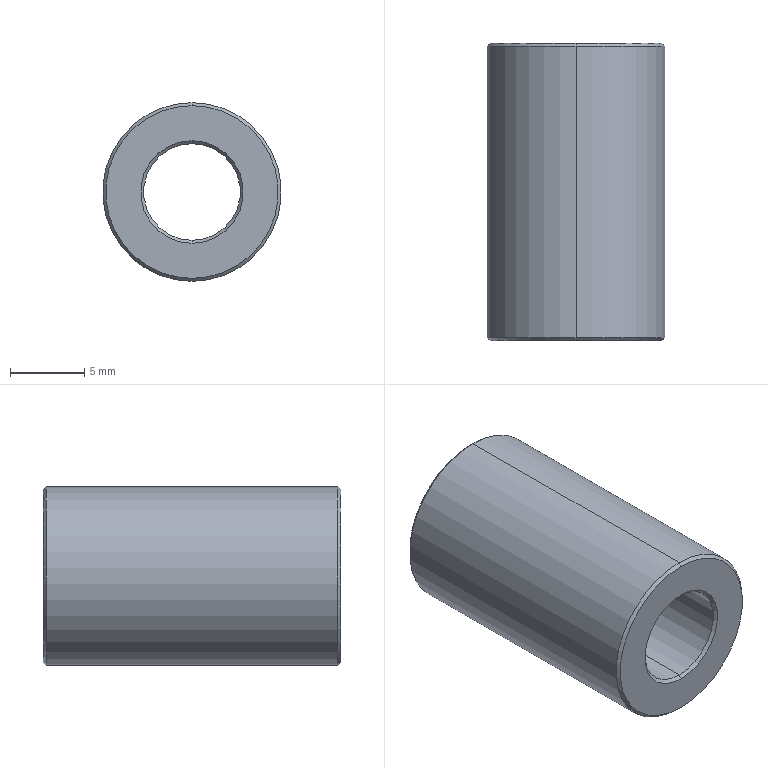Part | STEP file | PN_0025 lifting air cylinder extension rod_Default | 1 solid | 14 faces | box 12 x 20 x 12 mm | volume 1596 mm3 | cone 8 | cylinder 4 | plane 2 | commonest cylinder face diameters 6.5 x2 12 x2
STEP:
#1=CARTESIAN_POINT('',(0.,0.,0.));
#2=DIRECTION('',(0.,0.,1.));
#3=DIRECTION('',(1.,0.,0.));
#4=AXIS2_PLACEMENT_3D('',#1,#2,#3);
#5=CARTESIAN_POINT('',(0.,0.2,-3.25));
#6=VERTEX_POINT('',#5);
#7=CARTESIAN_POINT('',(0.,0.,-3.45));
#8=VERTEX_POINT('',#7);
#9=CARTESIAN_POINT('',(0.,0.,-3.45));
#10=DIRECTION('',(0.,-0.7071,-0.7071));
#11=VECTOR('',#10,1.);
#12=LINE('',#9,#11);
#13=CARTESIAN_POINT('',(0.,0.,0.));
#14=DIRECTION('',(0.,-1.,0.));
#15=DIRECTION('',(0.,0.,-1.));
#16=AXIS2_PLACEMENT_3D('',#13,#14,#15);
#17=CONICAL_SURFACE('',#16,3.45,0.7854);
#18=CARTESIAN_POINT('',(6.283,0.));
#19=DIRECTION('',(0.,1.));
#20=VECTOR('',#19,1.);
#21=LINE('',#18,#20);
#22=(GEOMETRIC_REPRESENTATION_CONTEXT(2)PARAMETRIC_REPRESENTATION_CONTEXT()REPRESENTATION_CONTEXT('',''));
#23=DEFINITIONAL_REPRESENTATION('',(#21),#22);
#24=PCURVE('',#17,#23);
#25=CARTESIAN_POINT('',(0.,0.,0.));
#26=DIRECTION('',(0.,-1.,0.));
#27=DIRECTION('',(0.,0.,-1.));
#28=AXIS2_PLACEMENT_3D('',#25,#26,#27);
#29=CONICAL_SURFACE('',#28,3.45,0.7854);
#30=CARTESIAN_POINT('',(0.,0.));
#31=DIRECTION('',(0.,1.));
#32=VECTOR('',#31,1.);
#33=LINE('',#30,#32);
#34=(GEOMETRIC_REPRESENTATION_CONTEXT(2)PARAMETRIC_REPRESENTATION_CONTEXT()REPRESENTATION_CONTEXT('',''));
#35=DEFINITIONAL_REPRESENTATION('',(#33),#34);
#36=PCURVE('',#29,#35);
#37=SURFACE_CURVE('',#12,(#24,#36),.PCURVE_S1.);
#38=EDGE_CURVE('',#6,#8,#37,.T.);
#39=ORIENTED_EDGE('',*,*,#38,.T.);
#40=CARTESIAN_POINT('',(0.,0.,3.45));
#41=VERTEX_POINT('',#40);
#42=CARTESIAN_POINT('',(0.,0.,0.));
#43=DIRECTION('',(0.,1.,0.));
#44=DIRECTION('',(0.,0.,1.));
#45=AXIS2_PLACEMENT_3D('',#42,#43,#44);
#46=CIRCLE('',#45,3.45);
#47=CARTESIAN_POINT('',(9.425,0.));
#48=DIRECTION('',(-1.,0.));
#49=VECTOR('',#48,1.);
#50=LINE('',#47,#49);
#51=(GEOMETRIC_REPRESENTATION_CONTEXT(2)PARAMETRIC_REPRESENTATION_CONTEXT()REPRESENTATION_CONTEXT('',''));
#52=DEFINITIONAL_REPRESENTATION('',(#50),#51);
#53=PCURVE('',#17,#52);
#54=CARTESIAN_POINT('',(0.,0.,0.));
#55=DIRECTION('',(0.,1.,0.));
#56=DIRECTION('',(0.,0.,1.));
#57=AXIS2_PLACEMENT_3D('',#54,#55,#56);
#58=PLANE('',#57);
#59=CARTESIAN_POINT('',(0.,0.));
#60=DIRECTION('',(1.,0.));
#61=AXIS2_PLACEMENT_2D('',#59,#60);
#62=CIRCLE('',#61,3.45);
#63=(GEOMETRIC_REPRESENTATION_CONTEXT(2)PARAMETRIC_REPRESENTATION_CONTEXT()REPRESENTATION_CONTEXT('',''));
#64=DEFINITIONAL_REPRESENTATION('',(#62),#63);
#65=PCURVE('',#58,#64);
#66=SURFACE_CURVE('',#46,(#53,#65),.PCURVE_S1.);
#67=EDGE_CURVE('',#8,#41,#66,.T.);
#68=ORIENTED_EDGE('',*,*,#67,.T.);
#69=CARTESIAN_POINT('',(0.,0.2,3.25));
#70=VERTEX_POINT('',#69);
#71=CARTESIAN_POINT('',(0.,0.,3.45));
#72=DIRECTION('',(0.,-0.7071,0.7071));
#73=VECTOR('',#72,1.);
#74=LINE('',#71,#73);
#75=CARTESIAN_POINT('',(3.142,0.));
#76=DIRECTION('',(0.,1.));
#77=VECTOR('',#76,1.);
#78=LINE('',#75,#77);
#79=(GEOMETRIC_REPRESENTATION_CONTEXT(2)PARAMETRIC_REPRESENTATION_CONTEXT()REPRESENTATION_CONTEXT('',''));
#80=DEFINITIONAL_REPRESENTATION('',(#78),#79);
#81=PCURVE('',#17,#80);
#82=CARTESIAN_POINT('',(3.142,0.));
#83=DIRECTION('',(0.,1.));
#84=VECTOR('',#83,1.);
#85=LINE('',#82,#84);
#86=(GEOMETRIC_REPRESENTATION_CONTEXT(2)PARAMETRIC_REPRESENTATION_CONTEXT()REPRESENTATION_CONTEXT('',''));
#87=DEFINITIONAL_REPRESENTATION('',(#85),#86);
#88=PCURVE('',#29,#87);
#89=SURFACE_CURVE('',#74,(#81,#88),.PCURVE_S1.);
#90=EDGE_CURVE('',#70,#41,#89,.T.);
#91=ORIENTED_EDGE('',*,*,#90,.F.);
#92=CARTESIAN_POINT('',(0.,0.2,0.));
#93=DIRECTION('',(0.,-1.,0.));
#94=DIRECTION('',(0.,0.,1.));
#95=AXIS2_PLACEMENT_3D('',#92,#93,#94);
#96=CIRCLE('',#95,3.25);
#97=CARTESIAN_POINT('',(3.142,-0.2));
#98=DIRECTION('',(1.,0.));
#99=VECTOR('',#98,1.);
#100=LINE('',#97,#99);
#101=(GEOMETRIC_REPRESENTATION_CONTEXT(2)PARAMETRIC_REPRESENTATION_CONTEXT()REPRESENTATION_CONTEXT('',''));
#102=DEFINITIONAL_REPRESENTATION('',(#100),#101);
#103=PCURVE('',#17,#102);
#104=CARTESIAN_POINT('',(0.,20.,0.));
#105=DIRECTION('',(0.,-1.,0.));
#106=DIRECTION('',(0.,0.,-1.));
#107=AXIS2_PLACEMENT_3D('',#104,#105,#106);
#108=CYLINDRICAL_SURFACE('',#107,3.25);
#109=CARTESIAN_POINT('',(3.142,19.8));
#110=DIRECTION('',(1.,0.));
#111=VECTOR('',#110,1.);
#112=LINE('',#109,#111);
#113=(GEOMETRIC_REPRESENTATION_CONTEXT(2)PARAMETRIC_REPRESENTATION_CONTEXT()REPRESENTATION_CONTEXT('',''));
#114=DEFINITIONAL_REPRESENTATION('',(#112),#113);
#115=PCURVE('',#108,#114);
#116=SURFACE_CURVE('',#96,(#103,#115),.PCURVE_S1.);
#117=EDGE_CURVE('',#70,#6,#116,.T.);
#118=ORIENTED_EDGE('',*,*,#117,.T.);
#119=EDGE_LOOP('',(#39,#68,#91,#118));
#120=FACE_BOUND('',#119,.F.);
#121=ADVANCED_FACE('',(#120),#17,.F.);
#122=CARTESIAN_POINT('',(0.,19.8,3.25));
#123=VERTEX_POINT('',#122);
#124=CARTESIAN_POINT('',(0.,20.,3.45));
#125=VERTEX_POINT('',#124);
#126=CARTESIAN_POINT('',(0.,19.8,3.25));
#127=DIRECTION('',(0.,0.7071,0.7071));
#128=VECTOR('',#127,1.);
#129=LINE('',#126,#128);
#130=CARTESIAN_POINT('',(0.,19.8,0.));
#131=DIRECTION('',(0.,1.,0.));
#132=DIRECTION('',(0.,0.,1.));
#133=AXIS2_PLACEMENT_3D('',#130,#131,#132);
#134=CONICAL_SURFACE('',#133,3.25,0.7854);
#135=CARTESIAN_POINT('',(6.283,0.));
#136=DIRECTION('',(0.,1.));
#137=VECTOR('',#136,1.);
#138=LINE('',#135,#137);
#139=(GEOMETRIC_REPRESENTATION_CONTEXT(2)PARAMETRIC_REPRESENTATION_CONTEXT()REPRESENTATION_CONTEXT('',''));
#140=DEFINITIONAL_REPRESENTATION('',(#138),#139);
#141=PCURVE('',#134,#140);
#142=CARTESIAN_POINT('',(0.,19.8,0.));
#143=DIRECTION('',(0.,1.,0.));
#144=DIRECTION('',(0.,0.,1.));
#145=AXIS2_PLACEMENT_3D('',#142,#143,#144);
#146=CONICAL_SURFACE('',#145,3.25,0.7854);
#147=CARTESIAN_POINT('',(0.,0.));
#148=DIRECTION('',(0.,1.));
#149=VECTOR('',#148,1.);
#150=LINE('',#147,#149);
#151=(GEOMETRIC_REPRESENTATION_CONTEXT(2)PARAMETRIC_REPRESENTATION_CONTEXT()REPRESENTATION_CONTEXT('',''));
#152=DEFINITIONAL_REPRESENTATION('',(#150),#151);
#153=PCURVE('',#146,#152);
#154=SURFACE_CURVE('',#129,(#141,#153),.PCURVE_S1.);
#155=EDGE_CURVE('',#123,#125,#154,.T.);
#156=ORIENTED_EDGE('',*,*,#155,.T.);
#157=CARTESIAN_POINT('',(0.,20.,-3.45));
#158=VERTEX_POINT('',#157);
#159=CARTESIAN_POINT('',(0.,20.,0.));
#160=DIRECTION('',(0.,-1.,0.));
#161=DIRECTION('',(0.,0.,1.));
#162=AXIS2_PLACEMENT_3D('',#159,#160,#161);
#163=CIRCLE('',#162,3.45);
#164=CARTESIAN_POINT('',(6.283,0.2));
#165=DIRECTION('',(-1.,0.));
#166=VECTOR('',#165,1.);
#167=LINE('',#164,#166);
#168=(GEOMETRIC_REPRESENTATION_CONTEXT(2)PARAMETRIC_REPRESENTATION_CONTEXT()REPRESENTATION_CONTEXT('',''));
#169=DEFINITIONAL_REPRESENTATION('',(#167),#168);
#170=PCURVE('',#134,#169);
#171=CARTESIAN_POINT('',(0.,20.,0.));
#172=DIRECTION('',(0.,1.,0.));
#173=DIRECTION('',(0.,0.,1.));
#174=AXIS2_PLACEMENT_3D('',#171,#172,#173);
#175=PLANE('',#174);
#176=CARTESIAN_POINT('',(3.45,0.));
#177=CARTESIAN_POINT('',(3.45,-5.976));
#178=CARTESIAN_POINT('',(-1.725,-2.988));
#179=CARTESIAN_POINT('',(-6.9,0.));
#180=CARTESIAN_POINT('',(-1.725,2.988));
#181=CARTESIAN_POINT('',(3.45,5.976));
#182=CARTESIAN_POINT('',(3.45,0.));
#183=(BOUNDED_CURVE()B_SPLINE_CURVE(2,(#176,#177,#178,#179,#180,#181,#182),.UNSPECIFIED.,.T.,.F.)B_SPLINE_CURVE_WITH_KNOTS((1,2,2,2,2,1),(-2.094,0.,2.094,4.189,6.283,8.378),.UNSPECIFIED.)CURVE()GEOMETRIC_REPRESENTATION_ITEM()RATIONAL_B_SPLINE_CURVE((1.,0.5,1.,0.5,1.,0.5,1.))REPRESENTATION_ITEM(''));
#184=(GEOMETRIC_REPRESENTATION_CONTEXT(2)PARAMETRIC_REPRESENTATION_CONTEXT()REPRESENTATION_CONTEXT('',''));
#185=DEFINITIONAL_REPRESENTATION('',(#183),#184);
#186=PCURVE('',#175,#185);
#187=SURFACE_CURVE('',#163,(#170,#186),.PCURVE_S1.);
#188=EDGE_CURVE('',#125,#158,#187,.T.);
#189=ORIENTED_EDGE('',*,*,#188,.T.);
#190=CARTESIAN_POINT('',(0.,19.8,-3.25));
#191=VERTEX_POINT('',#190);
#192=CARTESIAN_POINT('',(0.,19.8,-3.25));
#193=DIRECTION('',(0.,0.7071,-0.7071));
#194=VECTOR('',#193,1.);
#195=LINE('',#192,#194);
#196=CARTESIAN_POINT('',(3.142,0.));
#197=DIRECTION('',(0.,1.));
#198=VECTOR('',#197,1.);
#199=LINE('',#196,#198);
#200=(GEOMETRIC_REPRESENTATION_CONTEXT(2)PARAMETRIC_REPRESENTATION_CONTEXT()REPRESENTATION_CONTEXT('',''));
#201=DEFINITIONAL_REPRESENTATION('',(#199),#200);
#202=PCURVE('',#134,#201);
#203=CARTESIAN_POINT('',(3.142,0.));
#204=DIRECTION('',(0.,1.));
#205=VECTOR('',#204,1.);
#206=LINE('',#203,#205);
#207=(GEOMETRIC_REPRESENTATION_CONTEXT(2)PARAMETRIC_REPRESENTATION_CONTEXT()REPRESENTATION_CONTEXT('',''));
#208=DEFINITIONAL_REPRESENTATION('',(#206),#207);
#209=PCURVE('',#146,#208);
#210=SURFACE_CURVE('',#195,(#202,#209),.PCURVE_S1.);
#211=EDGE_CURVE('',#191,#158,#210,.T.);
#212=ORIENTED_EDGE('',*,*,#211,.F.);
#213=CARTESIAN_POINT('',(0.,19.8,0.));
#214=DIRECTION('',(0.,1.,0.));
#215=DIRECTION('',(0.,0.,1.));
#216=AXIS2_PLACEMENT_3D('',#213,#214,#215);
#217=CIRCLE('',#216,3.25);
#218=CARTESIAN_POINT('',(0.,0.));
#219=DIRECTION('',(1.,0.));
#220=VECTOR('',#219,1.);
#221=LINE('',#218,#220);
#222=(GEOMETRIC_REPRESENTATION_CONTEXT(2)PARAMETRIC_REPRESENTATION_CONTEXT()REPRESENTATION_CONTEXT('',''));
#223=DEFINITIONAL_REPRESENTATION('',(#221),#222);
#224=PCURVE('',#134,#223);
#225=CARTESIAN_POINT('',(9.425,0.2));
#226=DIRECTION('',(-1.,0.));
#227=VECTOR('',#226,1.);
#228=LINE('',#225,#227);
#229=(GEOMETRIC_REPRESENTATION_CONTEXT(2)PARAMETRIC_REPRESENTATION_CONTEXT()REPRESENTATION_CONTEXT('',''));
#230=DEFINITIONAL_REPRESENTATION('',(#228),#229);
#231=PCURVE('',#108,#230);
#232=SURFACE_CURVE('',#217,(#224,#231),.PCURVE_S1.);
#233=EDGE_CURVE('',#191,#123,#232,.T.);
#234=ORIENTED_EDGE('',*,*,#233,.T.);
#235=EDGE_LOOP('',(#156,#189,#212,#234));
#236=FACE_BOUND('',#235,.F.);
#237=ADVANCED_FACE('',(#236),#134,.F.);
#238=CARTESIAN_POINT('',(0.,0.,-5.8));
#239=VERTEX_POINT('',#238);
#240=CARTESIAN_POINT('',(0.,0.,5.8));
#241=VERTEX_POINT('',#240);
#242=CARTESIAN_POINT('',(0.,0.,0.));
#243=DIRECTION('',(0.,-1.,0.));
#244=DIRECTION('',(0.,0.,1.));
#245=AXIS2_PLACEMENT_3D('',#242,#243,#244);
#246=CIRCLE('',#245,5.8);
#247=CARTESIAN_POINT('',(0.,0.2,0.));
#248=DIRECTION('',(0.,1.,0.));
#249=DIRECTION('',(0.,0.,1.));
#250=AXIS2_PLACEMENT_3D('',#247,#248,#249);
#251=CONICAL_SURFACE('',#250,6.,0.7854);
#252=CARTESIAN_POINT('',(6.283,-0.2));
#253=DIRECTION('',(-1.,0.));
#254=VECTOR('',#253,1.);
#255=LINE('',#252,#254);
#256=(GEOMETRIC_REPRESENTATION_CONTEXT(2)PARAMETRIC_REPRESENTATION_CONTEXT()REPRESENTATION_CONTEXT('',''));
#257=DEFINITIONAL_REPRESENTATION('',(#255),#256);
#258=PCURVE('',#251,#257);
#259=CARTESIAN_POINT('',(5.8,0.));
#260=CARTESIAN_POINT('',(5.8,-10.046));
#261=CARTESIAN_POINT('',(-2.9,-5.023));
#262=CARTESIAN_POINT('',(-11.6,0.));
#263=CARTESIAN_POINT('',(-2.9,5.023));
#264=CARTESIAN_POINT('',(5.8,10.046));
#265=CARTESIAN_POINT('',(5.8,0.));
#266=(BOUNDED_CURVE()B_SPLINE_CURVE(2,(#259,#260,#261,#262,#263,#264,#265),.UNSPECIFIED.,.T.,.F.)B_SPLINE_CURVE_WITH_KNOTS((1,2,2,2,2,1),(-2.094,0.,2.094,4.189,6.283,8.378),.UNSPECIFIED.)CURVE()GEOMETRIC_REPRESENTATION_ITEM()RATIONAL_B_SPLINE_CURVE((1.,0.5,1.,0.5,1.,0.5,1.))REPRESENTATION_ITEM(''));
#267=(GEOMETRIC_REPRESENTATION_CONTEXT(2)PARAMETRIC_REPRESENTATION_CONTEXT()REPRESENTATION_CONTEXT('',''));
#268=DEFINITIONAL_REPRESENTATION('',(#266),#267);
#269=PCURVE('',#58,#268);
#270=SURFACE_CURVE('',#246,(#258,#269),.PCURVE_S1.);
#271=EDGE_CURVE('',#239,#241,#270,.T.);
#272=ORIENTED_EDGE('',*,*,#271,.F.);
#273=CARTESIAN_POINT('',(0.,0.2,-6.));
#274=VERTEX_POINT('',#273);
#275=CARTESIAN_POINT('',(0.,0.2,-6.));
#276=DIRECTION('',(0.,0.7071,-0.7071));
#277=VECTOR('',#276,1.);
#278=LINE('',#275,#277);
#279=CARTESIAN_POINT('',(3.142,0.));
#280=DIRECTION('',(0.,1.));
#281=VECTOR('',#280,1.);
#282=LINE('',#279,#281);
#283=(GEOMETRIC_REPRESENTATION_CONTEXT(2)PARAMETRIC_REPRESENTATION_CONTEXT()REPRESENTATION_CONTEXT('',''));
#284=DEFINITIONAL_REPRESENTATION('',(#282),#283);
#285=PCURVE('',#251,#284);
#286=CARTESIAN_POINT('',(0.,0.2,0.));
#287=DIRECTION('',(0.,1.,0.));
#288=DIRECTION('',(0.,0.,1.));
#289=AXIS2_PLACEMENT_3D('',#286,#287,#288);
#290=CONICAL_SURFACE('',#289,6.,0.7854);
#291=CARTESIAN_POINT('',(3.142,0.));
#292=DIRECTION('',(0.,1.));
#293=VECTOR('',#292,1.);
#294=LINE('',#291,#293);
#295=(GEOMETRIC_REPRESENTATION_CONTEXT(2)PARAMETRIC_REPRESENTATION_CONTEXT()REPRESENTATION_CONTEXT('',''));
#296=DEFINITIONAL_REPRESENTATION('',(#294),#295);
#297=PCURVE('',#290,#296);
#298=SURFACE_CURVE('',#278,(#285,#297),.PCURVE_S1.);
#299=EDGE_CURVE('',#239,#274,#298,.T.);
#300=ORIENTED_EDGE('',*,*,#299,.T.);
#301=CARTESIAN_POINT('',(0.,0.2,6.));
#302=VERTEX_POINT('',#301);
#303=CARTESIAN_POINT('',(0.,0.2,0.));
#304=DIRECTION('',(0.,1.,0.));
#305=DIRECTION('',(0.,0.,1.));
#306=AXIS2_PLACEMENT_3D('',#303,#304,#305);
#307=CIRCLE('',#306,6.);
#308=CARTESIAN_POINT('',(0.,0.));
#309=DIRECTION('',(1.,0.));
#310=VECTOR('',#309,1.);
#311=LINE('',#308,#310);
#312=(GEOMETRIC_REPRESENTATION_CONTEXT(2)PARAMETRIC_REPRESENTATION_CONTEXT()REPRESENTATION_CONTEXT('',''));
#313=DEFINITIONAL_REPRESENTATION('',(#311),#312);
#314=PCURVE('',#251,#313);
#315=CARTESIAN_POINT('',(0.,20.,0.));
#316=DIRECTION('',(0.,-1.,0.));
#317=DIRECTION('',(0.,0.,-1.));
#318=AXIS2_PLACEMENT_3D('',#315,#316,#317);
#319=CYLINDRICAL_SURFACE('',#318,6.);
#320=CARTESIAN_POINT('',(3.142,19.8));
#321=DIRECTION('',(-1.,0.));
#322=VECTOR('',#321,1.);
#323=LINE('',#320,#322);
#324=(GEOMETRIC_REPRESENTATION_CONTEXT(2)PARAMETRIC_REPRESENTATION_CONTEXT()REPRESENTATION_CONTEXT('',''));
#325=DEFINITIONAL_REPRESENTATION('',(#323),#324);
#326=PCURVE('',#319,#325);
#327=SURFACE_CURVE('',#307,(#314,#326),.PCURVE_S1.);
#328=EDGE_CURVE('',#302,#274,#327,.T.);
#329=ORIENTED_EDGE('',*,*,#328,.F.);
#330=CARTESIAN_POINT('',(0.,0.2,6.));
#331=DIRECTION('',(0.,0.7071,0.7071));
#332=VECTOR('',#331,1.);
#333=LINE('',#330,#332);
#334=CARTESIAN_POINT('',(0.,0.));
#335=DIRECTION('',(0.,1.));
#336=VECTOR('',#335,1.);
#337=LINE('',#334,#336);
#338=(GEOMETRIC_REPRESENTATION_CONTEXT(2)PARAMETRIC_REPRESENTATION_CONTEXT()REPRESENTATION_CONTEXT('',''));
#339=DEFINITIONAL_REPRESENTATION('',(#337),#338);
#340=PCURVE('',#251,#339);
#341=CARTESIAN_POINT('',(6.283,0.));
#342=DIRECTION('',(0.,1.));
#343=VECTOR('',#342,1.);
#344=LINE('',#341,#343);
#345=(GEOMETRIC_REPRESENTATION_CONTEXT(2)PARAMETRIC_REPRESENTATION_CONTEXT()REPRESENTATION_CONTEXT('',''));
#346=DEFINITIONAL_REPRESENTATION('',(#344),#345);
#347=PCURVE('',#290,#346);
#348=SURFACE_CURVE('',#333,(#340,#347),.PCURVE_S1.);
#349=EDGE_CURVE('',#241,#302,#348,.T.);
#350=ORIENTED_EDGE('',*,*,#349,.F.);
#351=EDGE_LOOP('',(#272,#300,#329,#350));
#352=FACE_BOUND('',#351,.T.);
#353=ADVANCED_FACE('',(#352),#251,.T.);
#354=CARTESIAN_POINT('',(0.,20.,5.8));
#355=VERTEX_POINT('',#354);
#356=CARTESIAN_POINT('',(0.,20.,-5.8));
#357=VERTEX_POINT('',#356);
#358=CARTESIAN_POINT('',(0.,20.,0.));
#359=DIRECTION('',(0.,1.,0.));
#360=DIRECTION('',(0.,0.,1.));
#361=AXIS2_PLACEMENT_3D('',#358,#359,#360);
#362=CIRCLE('',#361,5.8);
#363=CARTESIAN_POINT('',(0.,20.,0.));
#364=DIRECTION('',(0.,-1.,0.));
#365=DIRECTION('',(0.,0.,-1.));
#366=AXIS2_PLACEMENT_3D('',#363,#364,#365);
#367=CONICAL_SURFACE('',#366,5.8,0.7854);
#368=CARTESIAN_POINT('',(3.142,0.));
#369=DIRECTION('',(-1.,0.));
#370=VECTOR('',#369,1.);
#371=LINE('',#368,#370);
#372=(GEOMETRIC_REPRESENTATION_CONTEXT(2)PARAMETRIC_REPRESENTATION_CONTEXT()REPRESENTATION_CONTEXT('',''));
#373=DEFINITIONAL_REPRESENTATION('',(#371),#372);
#374=PCURVE('',#367,#373);
#375=CARTESIAN_POINT('',(0.,0.));
#376=DIRECTION('',(1.,0.));
#377=AXIS2_PLACEMENT_2D('',#375,#376);
#378=CIRCLE('',#377,5.8);
#379=(GEOMETRIC_REPRESENTATION_CONTEXT(2)PARAMETRIC_REPRESENTATION_CONTEXT()REPRESENTATION_CONTEXT('',''));
#380=DEFINITIONAL_REPRESENTATION('',(#378),#379);
#381=PCURVE('',#175,#380);
#382=SURFACE_CURVE('',#362,(#374,#381),.PCURVE_S1.);
#383=EDGE_CURVE('',#355,#357,#382,.T.);
#384=ORIENTED_EDGE('',*,*,#383,.F.);
#385=CARTESIAN_POINT('',(0.,19.8,6.));
#386=VERTEX_POINT('',#385);
#387=CARTESIAN_POINT('',(0.,20.,5.8));
#388=DIRECTION('',(0.,-0.7071,0.7071));
#389=VECTOR('',#388,1.);
#390=LINE('',#387,#389);
#391=CARTESIAN_POINT('',(3.142,0.));
#392=DIRECTION('',(0.,1.));
#393=VECTOR('',#392,1.);
#394=LINE('',#391,#393);
#395=(GEOMETRIC_REPRESENTATION_CONTEXT(2)PARAMETRIC_REPRESENTATION_CONTEXT()REPRESENTATION_CONTEXT('',''));
#396=DEFINITIONAL_REPRESENTATION('',(#394),#395);
#397=PCURVE('',#367,#396);
#398=CARTESIAN_POINT('',(0.,20.,0.));
#399=DIRECTION('',(0.,-1.,0.));
#400=DIRECTION('',(0.,0.,-1.));
#401=AXIS2_PLACEMENT_3D('',#398,#399,#400);
#402=CONICAL_SURFACE('',#401,5.8,0.7854);
#403=CARTESIAN_POINT('',(3.142,0.));
#404=DIRECTION('',(0.,1.));
#405=VECTOR('',#404,1.);
#406=LINE('',#403,#405);
#407=(GEOMETRIC_REPRESENTATION_CONTEXT(2)PARAMETRIC_REPRESENTATION_CONTEXT()REPRESENTATION_CONTEXT('',''));
#408=DEFINITIONAL_REPRESENTATION('',(#406),#407);
#409=PCURVE('',#402,#408);
#410=SURFACE_CURVE('',#390,(#397,#409),.PCURVE_S1.);
#411=EDGE_CURVE('',#355,#386,#410,.T.);
#412=ORIENTED_EDGE('',*,*,#411,.T.);
#413=CARTESIAN_POINT('',(0.,19.8,-6.));
#414=VERTEX_POINT('',#413);
#415=CARTESIAN_POINT('',(0.,19.8,0.));
#416=DIRECTION('',(0.,-1.,0.));
#417=DIRECTION('',(0.,0.,1.));
#418=AXIS2_PLACEMENT_3D('',#415,#416,#417);
#419=CIRCLE('',#418,6.);
#420=CARTESIAN_POINT('',(-3.142,0.2));
#421=DIRECTION('',(1.,0.));
#422=VECTOR('',#421,1.);
#423=LINE('',#420,#422);
#424=(GEOMETRIC_REPRESENTATION_CONTEXT(2)PARAMETRIC_REPRESENTATION_CONTEXT()REPRESENTATION_CONTEXT('',''));
#425=DEFINITIONAL_REPRESENTATION('',(#423),#424);
#426=PCURVE('',#367,#425);
#427=CARTESIAN_POINT('',(-3.142,0.2));
#428=DIRECTION('',(1.,0.));
#429=VECTOR('',#428,1.);
#430=LINE('',#427,#429);
#431=(GEOMETRIC_REPRESENTATION_CONTEXT(2)PARAMETRIC_REPRESENTATION_CONTEXT()REPRESENTATION_CONTEXT('',''));
#432=DEFINITIONAL_REPRESENTATION('',(#430),#431);
#433=PCURVE('',#319,#432);
#434=SURFACE_CURVE('',#419,(#426,#433),.PCURVE_S1.);
#435=EDGE_CURVE('',#414,#386,#434,.T.);
#436=ORIENTED_EDGE('',*,*,#435,.F.);
#437=CARTESIAN_POINT('',(0.,20.,-5.8));
#438=DIRECTION('',(0.,-0.7071,-0.7071));
#439=VECTOR('',#438,1.);
#440=LINE('',#437,#439);
#441=CARTESIAN_POINT('',(0.,0.));
#442=DIRECTION('',(0.,1.));
#443=VECTOR('',#442,1.);
#444=LINE('',#441,#443);
#445=(GEOMETRIC_REPRESENTATION_CONTEXT(2)PARAMETRIC_REPRESENTATION_CONTEXT()REPRESENTATION_CONTEXT('',''));
#446=DEFINITIONAL_REPRESENTATION('',(#444),#445);
#447=PCURVE('',#367,#446);
#448=CARTESIAN_POINT('',(6.283,0.));
#449=DIRECTION('',(0.,1.));
#450=VECTOR('',#449,1.);
#451=LINE('',#448,#450);
#452=(GEOMETRIC_REPRESENTATION_CONTEXT(2)PARAMETRIC_REPRESENTATION_CONTEXT()REPRESENTATION_CONTEXT('',''));
#453=DEFINITIONAL_REPRESENTATION('',(#451),#452);
#454=PCURVE('',#402,#453);
#455=SURFACE_CURVE('',#440,(#447,#454),.PCURVE_S1.);
#456=EDGE_CURVE('',#357,#414,#455,.T.);
#457=ORIENTED_EDGE('',*,*,#456,.F.);
#458=EDGE_LOOP('',(#384,#412,#436,#457));
#459=FACE_BOUND('',#458,.T.);
#460=ADVANCED_FACE('',(#459),#367,.T.);
#461=CARTESIAN_POINT('',(0.,20.,-3.25));
#462=DIRECTION('',(0.,-1.,0.));
#463=VECTOR('',#462,1.);
#464=LINE('',#461,#463);
#465=CARTESIAN_POINT('',(6.283,0.));
#466=DIRECTION('',(0.,1.));
#467=VECTOR('',#466,1.);
#468=LINE('',#465,#467);
#469=(GEOMETRIC_REPRESENTATION_CONTEXT(2)PARAMETRIC_REPRESENTATION_CONTEXT()REPRESENTATION_CONTEXT('',''));
#470=DEFINITIONAL_REPRESENTATION('',(#468),#469);
#471=PCURVE('',#108,#470);
#472=CARTESIAN_POINT('',(0.,20.,0.));
#473=DIRECTION('',(0.,-1.,0.));
#474=DIRECTION('',(0.,0.,-1.));
#475=AXIS2_PLACEMENT_3D('',#472,#473,#474);
#476=CYLINDRICAL_SURFACE('',#475,3.25);
#477=CARTESIAN_POINT('',(0.,0.));
#478=DIRECTION('',(0.,1.));
#479=VECTOR('',#478,1.);
#480=LINE('',#477,#479);
#481=(GEOMETRIC_REPRESENTATION_CONTEXT(2)PARAMETRIC_REPRESENTATION_CONTEXT()REPRESENTATION_CONTEXT('',''));
#482=DEFINITIONAL_REPRESENTATION('',(#480),#481);
#483=PCURVE('',#476,#482);
#484=SURFACE_CURVE('',#464,(#471,#483),.PCURVE_S1.);
#485=EDGE_CURVE('',#191,#6,#484,.T.);
#486=ORIENTED_EDGE('',*,*,#485,.T.);
#487=ORIENTED_EDGE('',*,*,#117,.F.);
#488=CARTESIAN_POINT('',(0.,20.,3.25));
#489=DIRECTION('',(0.,-1.,0.));
#490=VECTOR('',#489,1.);
#491=LINE('',#488,#490);
#492=CARTESIAN_POINT('',(3.142,0.));
#493=DIRECTION('',(0.,1.));
#494=VECTOR('',#493,1.);
#495=LINE('',#492,#494);
#496=(GEOMETRIC_REPRESENTATION_CONTEXT(2)PARAMETRIC_REPRESENTATION_CONTEXT()REPRESENTATION_CONTEXT('',''));
#497=DEFINITIONAL_REPRESENTATION('',(#495),#496);
#498=PCURVE('',#108,#497);
#499=CARTESIAN_POINT('',(3.142,0.));
#500=DIRECTION('',(0.,1.));
#501=VECTOR('',#500,1.);
#502=LINE('',#499,#501);
#503=(GEOMETRIC_REPRESENTATION_CONTEXT(2)PARAMETRIC_REPRESENTATION_CONTEXT()REPRESENTATION_CONTEXT('',''));
#504=DEFINITIONAL_REPRESENTATION('',(#502),#503);
#505=PCURVE('',#476,#504);
#506=SURFACE_CURVE('',#491,(#498,#505),.PCURVE_S1.);
#507=EDGE_CURVE('',#123,#70,#506,.T.);
#508=ORIENTED_EDGE('',*,*,#507,.F.);
#509=ORIENTED_EDGE('',*,*,#233,.F.);
#510=EDGE_LOOP('',(#486,#487,#508,#509));
#511=FACE_BOUND('',#510,.F.);
#512=ADVANCED_FACE('',(#511),#108,.F.);
#513=ORIENTED_EDGE('',*,*,#435,.T.);
#514=CARTESIAN_POINT('',(0.,20.,6.));
#515=DIRECTION('',(0.,-1.,0.));
#516=VECTOR('',#515,1.);
#517=LINE('',#514,#516);
#518=CARTESIAN_POINT('',(3.142,0.));
#519=DIRECTION('',(0.,1.));
#520=VECTOR('',#519,1.);
#521=LINE('',#518,#520);
#522=(GEOMETRIC_REPRESENTATION_CONTEXT(2)PARAMETRIC_REPRESENTATION_CONTEXT()REPRESENTATION_CONTEXT('',''));
#523=DEFINITIONAL_REPRESENTATION('',(#521),#522);
#524=PCURVE('',#319,#523);
#525=CARTESIAN_POINT('',(0.,20.,0.));
#526=DIRECTION('',(0.,-1.,0.));
#527=DIRECTION('',(0.,0.,-1.));
#528=AXIS2_PLACEMENT_3D('',#525,#526,#527);
#529=CYLINDRICAL_SURFACE('',#528,6.);
#530=CARTESIAN_POINT('',(3.142,0.));
#531=DIRECTION('',(0.,1.));
#532=VECTOR('',#531,1.);
#533=LINE('',#530,#532);
#534=(GEOMETRIC_REPRESENTATION_CONTEXT(2)PARAMETRIC_REPRESENTATION_CONTEXT()REPRESENTATION_CONTEXT('',''));
#535=DEFINITIONAL_REPRESENTATION('',(#533),#534);
#536=PCURVE('',#529,#535);
#537=SURFACE_CURVE('',#517,(#524,#536),.PCURVE_S1.);
#538=EDGE_CURVE('',#386,#302,#537,.T.);
#539=ORIENTED_EDGE('',*,*,#538,.T.);
#540=ORIENTED_EDGE('',*,*,#328,.T.);
#541=CARTESIAN_POINT('',(0.,20.,-6.));
#542=DIRECTION('',(0.,-1.,0.));
#543=VECTOR('',#542,1.);
#544=LINE('',#541,#543);
#545=CARTESIAN_POINT('',(0.,0.));
#546=DIRECTION('',(0.,1.));
#547=VECTOR('',#546,1.);
#548=LINE('',#545,#547);
#549=(GEOMETRIC_REPRESENTATION_CONTEXT(2)PARAMETRIC_REPRESENTATION_CONTEXT()REPRESENTATION_CONTEXT('',''));
#550=DEFINITIONAL_REPRESENTATION('',(#548),#549);
#551=PCURVE('',#319,#550);
#552=CARTESIAN_POINT('',(6.283,0.));
#553=DIRECTION('',(0.,1.));
#554=VECTOR('',#553,1.);
#555=LINE('',#552,#554);
#556=(GEOMETRIC_REPRESENTATION_CONTEXT(2)PARAMETRIC_REPRESENTATION_CONTEXT()REPRESENTATION_CONTEXT('',''));
#557=DEFINITIONAL_REPRESENTATION('',(#555),#556);
#558=PCURVE('',#529,#557);
#559=SURFACE_CURVE('',#544,(#551,#558),.PCURVE_S1.);
#560=EDGE_CURVE('',#414,#274,#559,.T.);
#561=ORIENTED_EDGE('',*,*,#560,.F.);
#562=EDGE_LOOP('',(#513,#539,#540,#561));
#563=FACE_BOUND('',#562,.T.);
#564=ADVANCED_FACE('',(#563),#319,.T.);
#565=CARTESIAN_POINT('',(0.,20.,0.));
#566=DIRECTION('',(0.,1.,0.));
#567=DIRECTION('',(0.,0.,1.));
#568=AXIS2_PLACEMENT_3D('',#565,#566,#567);
#569=CIRCLE('',#568,5.8);
#570=CARTESIAN_POINT('',(0.,0.));
#571=DIRECTION('',(1.,0.));
#572=AXIS2_PLACEMENT_2D('',#570,#571);
#573=CIRCLE('',#572,5.8);
#574=(GEOMETRIC_REPRESENTATION_CONTEXT(2)PARAMETRIC_REPRESENTATION_CONTEXT()REPRESENTATION_CONTEXT('',''));
#575=DEFINITIONAL_REPRESENTATION('',(#573),#574);
#576=PCURVE('',#175,#575);
#577=CARTESIAN_POINT('',(9.425,0.));
#578=DIRECTION('',(-1.,0.));
#579=VECTOR('',#578,1.);
#580=LINE('',#577,#579);
#581=(GEOMETRIC_REPRESENTATION_CONTEXT(2)PARAMETRIC_REPRESENTATION_CONTEXT()REPRESENTATION_CONTEXT('',''));
#582=DEFINITIONAL_REPRESENTATION('',(#580),#581);
#583=PCURVE('',#402,#582);
#584=SURFACE_CURVE('',#569,(#576,#583),.PCURVE_S1.);
#585=EDGE_CURVE('',#357,#355,#584,.T.);
#586=ORIENTED_EDGE('',*,*,#585,.T.);
#587=ORIENTED_EDGE('',*,*,#383,.T.);
#588=EDGE_LOOP('',(#586,#587));
#589=FACE_BOUND('',#588,.T.);
#590=ORIENTED_EDGE('',*,*,#188,.T.);
#591=CARTESIAN_POINT('',(0.,20.,0.));
#592=DIRECTION('',(0.,-1.,0.));
#593=DIRECTION('',(0.,0.,1.));
#594=AXIS2_PLACEMENT_3D('',#591,#592,#593);
#595=CIRCLE('',#594,3.45);
#596=CARTESIAN_POINT('',(3.45,0.));
#597=CARTESIAN_POINT('',(3.45,-5.976));
#598=CARTESIAN_POINT('',(-1.725,-2.988));
#599=CARTESIAN_POINT('',(-6.9,0.));
#600=CARTESIAN_POINT('',(-1.725,2.988));
#601=CARTESIAN_POINT('',(3.45,5.976));
#602=CARTESIAN_POINT('',(3.45,0.));
#603=(BOUNDED_CURVE()B_SPLINE_CURVE(2,(#596,#597,#598,#599,#600,#601,#602),.UNSPECIFIED.,.T.,.F.)B_SPLINE_CURVE_WITH_KNOTS((1,2,2,2,2,1),(-2.094,0.,2.094,4.189,6.283,8.378),.UNSPECIFIED.)CURVE()GEOMETRIC_REPRESENTATION_ITEM()RATIONAL_B_SPLINE_CURVE((1.,0.5,1.,0.5,1.,0.5,1.))REPRESENTATION_ITEM(''));
#604=(GEOMETRIC_REPRESENTATION_CONTEXT(2)PARAMETRIC_REPRESENTATION_CONTEXT()REPRESENTATION_CONTEXT('',''));
#605=DEFINITIONAL_REPRESENTATION('',(#603),#604);
#606=PCURVE('',#175,#605);
#607=CARTESIAN_POINT('',(6.283,0.2));
#608=DIRECTION('',(-1.,0.));
#609=VECTOR('',#608,1.);
#610=LINE('',#607,#609);
#611=(GEOMETRIC_REPRESENTATION_CONTEXT(2)PARAMETRIC_REPRESENTATION_CONTEXT()REPRESENTATION_CONTEXT('',''));
#612=DEFINITIONAL_REPRESENTATION('',(#610),#611);
#613=PCURVE('',#146,#612);
#614=SURFACE_CURVE('',#595,(#606,#613),.PCURVE_S1.);
#615=EDGE_CURVE('',#158,#125,#614,.T.);
#616=ORIENTED_EDGE('',*,*,#615,.T.);
#617=EDGE_LOOP('',(#590,#616));
#618=FACE_BOUND('',#617,.T.);
#619=ADVANCED_FACE('',(#589,#618),#175,.T.);
#620=CARTESIAN_POINT('',(0.,0.,0.));
#621=DIRECTION('',(0.,-1.,0.));
#622=DIRECTION('',(0.,0.,1.));
#623=AXIS2_PLACEMENT_3D('',#620,#621,#622);
#624=CIRCLE('',#623,5.8);
#625=CARTESIAN_POINT('',(5.8,0.));
#626=CARTESIAN_POINT('',(5.8,-10.046));
#627=CARTESIAN_POINT('',(-2.9,-5.023));
#628=CARTESIAN_POINT('',(-11.6,0.));
#629=CARTESIAN_POINT('',(-2.9,5.023));
#630=CARTESIAN_POINT('',(5.8,10.046));
#631=CARTESIAN_POINT('',(5.8,0.));
#632=(BOUNDED_CURVE()B_SPLINE_CURVE(2,(#625,#626,#627,#628,#629,#630,#631),.UNSPECIFIED.,.T.,.F.)B_SPLINE_CURVE_WITH_KNOTS((1,2,2,2,2,1),(-2.094,0.,2.094,4.189,6.283,8.378),.UNSPECIFIED.)CURVE()GEOMETRIC_REPRESENTATION_ITEM()RATIONAL_B_SPLINE_CURVE((1.,0.5,1.,0.5,1.,0.5,1.))REPRESENTATION_ITEM(''));
#633=(GEOMETRIC_REPRESENTATION_CONTEXT(2)PARAMETRIC_REPRESENTATION_CONTEXT()REPRESENTATION_CONTEXT('',''));
#634=DEFINITIONAL_REPRESENTATION('',(#632),#633);
#635=PCURVE('',#58,#634);
#636=CARTESIAN_POINT('',(6.283,-0.2));
#637=DIRECTION('',(-1.,0.));
#638=VECTOR('',#637,1.);
#639=LINE('',#636,#638);
#640=(GEOMETRIC_REPRESENTATION_CONTEXT(2)PARAMETRIC_REPRESENTATION_CONTEXT()REPRESENTATION_CONTEXT('',''));
#641=DEFINITIONAL_REPRESENTATION('',(#639),#640);
#642=PCURVE('',#290,#641);
#643=SURFACE_CURVE('',#624,(#635,#642),.PCURVE_S1.);
#644=EDGE_CURVE('',#241,#239,#643,.T.);
#645=ORIENTED_EDGE('',*,*,#644,.T.);
#646=ORIENTED_EDGE('',*,*,#271,.T.);
#647=EDGE_LOOP('',(#645,#646));
#648=FACE_BOUND('',#647,.T.);
#649=ORIENTED_EDGE('',*,*,#67,.T.);
#650=CARTESIAN_POINT('',(0.,0.,0.));
#651=DIRECTION('',(0.,1.,0.));
#652=DIRECTION('',(0.,0.,1.));
#653=AXIS2_PLACEMENT_3D('',#650,#651,#652);
#654=CIRCLE('',#653,3.45);
#655=CARTESIAN_POINT('',(0.,0.));
#656=DIRECTION('',(1.,0.));
#657=AXIS2_PLACEMENT_2D('',#655,#656);
#658=CIRCLE('',#657,3.45);
#659=(GEOMETRIC_REPRESENTATION_CONTEXT(2)PARAMETRIC_REPRESENTATION_CONTEXT()REPRESENTATION_CONTEXT('',''));
#660=DEFINITIONAL_REPRESENTATION('',(#658),#659);
#661=PCURVE('',#58,#660);
#662=CARTESIAN_POINT('',(3.142,0.));
#663=DIRECTION('',(-1.,0.));
#664=VECTOR('',#663,1.);
#665=LINE('',#662,#664);
#666=(GEOMETRIC_REPRESENTATION_CONTEXT(2)PARAMETRIC_REPRESENTATION_CONTEXT()REPRESENTATION_CONTEXT('',''));
#667=DEFINITIONAL_REPRESENTATION('',(#665),#666);
#668=PCURVE('',#29,#667);
#669=SURFACE_CURVE('',#654,(#661,#668),.PCURVE_S1.);
#670=EDGE_CURVE('',#41,#8,#669,.T.);
#671=ORIENTED_EDGE('',*,*,#670,.T.);
#672=EDGE_LOOP('',(#649,#671));
#673=FACE_BOUND('',#672,.T.);
#674=ADVANCED_FACE('',(#648,#673),#58,.F.);
#675=ORIENTED_EDGE('',*,*,#538,.F.);
#676=CARTESIAN_POINT('',(0.,19.8,0.));
#677=DIRECTION('',(0.,-1.,0.));
#678=DIRECTION('',(0.,0.,1.));
#679=AXIS2_PLACEMENT_3D('',#676,#677,#678);
#680=CIRCLE('',#679,6.);
#681=CARTESIAN_POINT('',(3.142,0.2));
#682=DIRECTION('',(1.,0.));
#683=VECTOR('',#682,1.);
#684=LINE('',#681,#683);
#685=(GEOMETRIC_REPRESENTATION_CONTEXT(2)PARAMETRIC_REPRESENTATION_CONTEXT()REPRESENTATION_CONTEXT('',''));
#686=DEFINITIONAL_REPRESENTATION('',(#684),#685);
#687=PCURVE('',#529,#686);
#688=CARTESIAN_POINT('',(3.142,0.2));
#689=DIRECTION('',(1.,0.));
#690=VECTOR('',#689,1.);
#691=LINE('',#688,#690);
#692=(GEOMETRIC_REPRESENTATION_CONTEXT(2)PARAMETRIC_REPRESENTATION_CONTEXT()REPRESENTATION_CONTEXT('',''));
#693=DEFINITIONAL_REPRESENTATION('',(#691),#692);
#694=PCURVE('',#402,#693);
#695=SURFACE_CURVE('',#680,(#687,#694),.PCURVE_S1.);
#696=EDGE_CURVE('',#386,#414,#695,.T.);
#697=ORIENTED_EDGE('',*,*,#696,.T.);
#698=ORIENTED_EDGE('',*,*,#560,.T.);
#699=CARTESIAN_POINT('',(0.,0.2,0.));
#700=DIRECTION('',(0.,1.,0.));
#701=DIRECTION('',(0.,0.,1.));
#702=AXIS2_PLACEMENT_3D('',#699,#700,#701);
#703=CIRCLE('',#702,6.);
#704=CARTESIAN_POINT('',(9.425,19.8));
#705=DIRECTION('',(-1.,0.));
#706=VECTOR('',#705,1.);
#707=LINE('',#704,#706);
#708=(GEOMETRIC_REPRESENTATION_CONTEXT(2)PARAMETRIC_REPRESENTATION_CONTEXT()REPRESENTATION_CONTEXT('',''));
#709=DEFINITIONAL_REPRESENTATION('',(#707),#708);
#710=PCURVE('',#529,#709);
#711=CARTESIAN_POINT('',(0.,0.));
#712=DIRECTION('',(1.,0.));
#713=VECTOR('',#712,1.);
#714=LINE('',#711,#713);
#715=(GEOMETRIC_REPRESENTATION_CONTEXT(2)PARAMETRIC_REPRESENTATION_CONTEXT()REPRESENTATION_CONTEXT('',''));
#716=DEFINITIONAL_REPRESENTATION('',(#714),#715);
#717=PCURVE('',#290,#716);
#718=SURFACE_CURVE('',#703,(#710,#717),.PCURVE_S1.);
#719=EDGE_CURVE('',#274,#302,#718,.T.);
#720=ORIENTED_EDGE('',*,*,#719,.T.);
#721=EDGE_LOOP('',(#675,#697,#698,#720));
#722=FACE_BOUND('',#721,.T.);
#723=ADVANCED_FACE('',(#722),#529,.T.);
#724=CARTESIAN_POINT('',(0.,0.2,0.));
#725=DIRECTION('',(0.,-1.,0.));
#726=DIRECTION('',(0.,0.,1.));
#727=AXIS2_PLACEMENT_3D('',#724,#725,#726);
#728=CIRCLE('',#727,3.25);
#729=CARTESIAN_POINT('',(-3.142,19.8));
#730=DIRECTION('',(1.,0.));
#731=VECTOR('',#730,1.);
#732=LINE('',#729,#731);
#733=(GEOMETRIC_REPRESENTATION_CONTEXT(2)PARAMETRIC_REPRESENTATION_CONTEXT()REPRESENTATION_CONTEXT('',''));
#734=DEFINITIONAL_REPRESENTATION('',(#732),#733);
#735=PCURVE('',#476,#734);
#736=CARTESIAN_POINT('',(-3.142,-0.2));
#737=DIRECTION('',(1.,0.));
#738=VECTOR('',#737,1.);
#739=LINE('',#736,#738);
#740=(GEOMETRIC_REPRESENTATION_CONTEXT(2)PARAMETRIC_REPRESENTATION_CONTEXT()REPRESENTATION_CONTEXT('',''));
#741=DEFINITIONAL_REPRESENTATION('',(#739),#740);
#742=PCURVE('',#29,#741);
#743=SURFACE_CURVE('',#728,(#735,#742),.PCURVE_S1.);
#744=EDGE_CURVE('',#6,#70,#743,.T.);
#745=ORIENTED_EDGE('',*,*,#744,.F.);
#746=ORIENTED_EDGE('',*,*,#485,.F.);
#747=CARTESIAN_POINT('',(0.,19.8,0.));
#748=DIRECTION('',(0.,1.,0.));
#749=DIRECTION('',(0.,0.,1.));
#750=AXIS2_PLACEMENT_3D('',#747,#748,#749);
#751=CIRCLE('',#750,3.25);
#752=CARTESIAN_POINT('',(3.142,0.2));
#753=DIRECTION('',(-1.,0.));
#754=VECTOR('',#753,1.);
#755=LINE('',#752,#754);
#756=(GEOMETRIC_REPRESENTATION_CONTEXT(2)PARAMETRIC_REPRESENTATION_CONTEXT()REPRESENTATION_CONTEXT('',''));
#757=DEFINITIONAL_REPRESENTATION('',(#755),#756);
#758=PCURVE('',#476,#757);
#759=CARTESIAN_POINT('',(0.,0.));
#760=DIRECTION('',(1.,0.));
#761=VECTOR('',#760,1.);
#762=LINE('',#759,#761);
#763=(GEOMETRIC_REPRESENTATION_CONTEXT(2)PARAMETRIC_REPRESENTATION_CONTEXT()REPRESENTATION_CONTEXT('',''));
#764=DEFINITIONAL_REPRESENTATION('',(#762),#763);
#765=PCURVE('',#146,#764);
#766=SURFACE_CURVE('',#751,(#758,#765),.PCURVE_S1.);
#767=EDGE_CURVE('',#123,#191,#766,.T.);
#768=ORIENTED_EDGE('',*,*,#767,.F.);
#769=ORIENTED_EDGE('',*,*,#507,.T.);
#770=EDGE_LOOP('',(#745,#746,#768,#769));
#771=FACE_BOUND('',#770,.F.);
#772=ADVANCED_FACE('',(#771),#476,.F.);
#773=ORIENTED_EDGE('',*,*,#411,.F.);
#774=ORIENTED_EDGE('',*,*,#585,.F.);
#775=ORIENTED_EDGE('',*,*,#456,.T.);
#776=ORIENTED_EDGE('',*,*,#696,.F.);
#777=EDGE_LOOP('',(#773,#774,#775,#776));
#778=FACE_BOUND('',#777,.T.);
#779=ADVANCED_FACE('',(#778),#402,.T.);
#780=ORIENTED_EDGE('',*,*,#299,.F.);
#781=ORIENTED_EDGE('',*,*,#644,.F.);
#782=ORIENTED_EDGE('',*,*,#349,.T.);
#783=ORIENTED_EDGE('',*,*,#719,.F.);
#784=EDGE_LOOP('',(#780,#781,#782,#783));
#785=FACE_BOUND('',#784,.T.);
#786=ADVANCED_FACE('',(#785),#290,.T.);
#787=ORIENTED_EDGE('',*,*,#615,.T.);
#788=ORIENTED_EDGE('',*,*,#155,.F.);
#789=ORIENTED_EDGE('',*,*,#767,.T.);
#790=ORIENTED_EDGE('',*,*,#211,.T.);
#791=EDGE_LOOP('',(#787,#788,#789,#790));
#792=FACE_BOUND('',#791,.F.);
#793=ADVANCED_FACE('',(#792),#146,.F.);
#794=ORIENTED_EDGE('',*,*,#670,.T.);
#795=ORIENTED_EDGE('',*,*,#38,.F.);
#796=ORIENTED_EDGE('',*,*,#744,.T.);
#797=ORIENTED_EDGE('',*,*,#90,.T.);
#798=EDGE_LOOP('',(#794,#795,#796,#797));
#799=FACE_BOUND('',#798,.F.);
#800=ADVANCED_FACE('',(#799),#29,.F.);
#801=CLOSED_SHELL('',(#121,#237,#353,#460,#512,#564,#619,#674,#723,#772,#779,#786,#793,#800));
#802=MANIFOLD_SOLID_BREP('',#801);
#803=(LENGTH_UNIT()NAMED_UNIT(*)SI_UNIT(.MILLI.,.METRE.));
#804=UNCERTAINTY_MEASURE_WITH_UNIT(LENGTH_MEASURE(0.0000001),#803,'','');
#805=(NAMED_UNIT(*)PLANE_ANGLE_UNIT()SI_UNIT($,.RADIAN.));
#806=(NAMED_UNIT(*)SI_UNIT($,.STERADIAN.)SOLID_ANGLE_UNIT());
#807=(GEOMETRIC_REPRESENTATION_CONTEXT(3)GLOBAL_UNCERTAINTY_ASSIGNED_CONTEXT((#804))GLOBAL_UNIT_ASSIGNED_CONTEXT((#803,#805,#806))REPRESENTATION_CONTEXT('',''));
#808=ADVANCED_BREP_SHAPE_REPRESENTATION('',(#4,#802),#807);